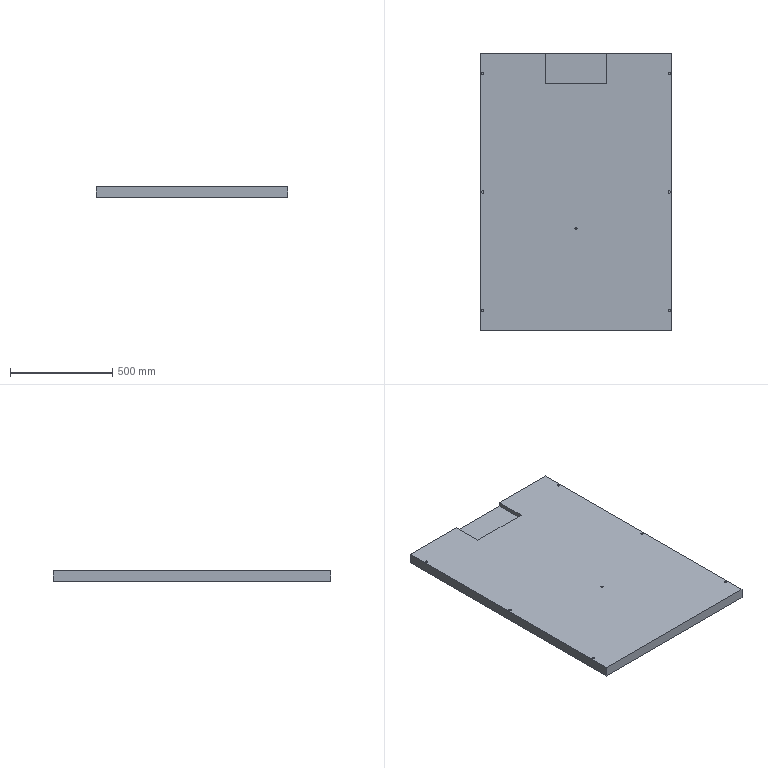Part | SolidWorks | features ICE 2, Extrusion 1 | 1 solid | 31 faces | box 940 x 1360 x 50 mm | volume 63007025 mm3 | plane 17 | cylinder 14 | commonest cylinder face diameters 11 x12 10 x2
STEP:
#1=CARTESIAN_POINT('',(-463.,-580.,30.));
#2=VERTEX_POINT('',#1);
#3=CARTESIAN_POINT('',(-452.,-580.,30.));
#4=VERTEX_POINT('',#3);
#5=CARTESIAN_POINT('',(-457.5,-580.,30.));
#6=DIRECTION('',(0.,0.,1.));
#7=DIRECTION('',(-1.,0.,0.));
#8=AXIS2_PLACEMENT_3D('',#5,#6,#7);
#9=CIRCLE('',#8,5.5);
#10=EDGE_CURVE('',#2,#4,#9,.T.);
#11=ORIENTED_EDGE('',*,*,#10,.F.);
#12=CARTESIAN_POINT('',(-463.,-580.,50.));
#13=VERTEX_POINT('',#12);
#14=CARTESIAN_POINT('',(-463.,-580.,30.));
#15=DIRECTION('',(0.,0.,1.));
#16=VECTOR('',#15,1000.);
#17=LINE('',#14,#16);
#18=EDGE_CURVE('',#2,#13,#17,.T.);
#19=ORIENTED_EDGE('',*,*,#18,.T.);
#20=CARTESIAN_POINT('',(-452.,-580.,50.));
#21=VERTEX_POINT('',#20);
#22=CARTESIAN_POINT('',(-457.5,-580.,50.));
#23=DIRECTION('',(0.,0.,1.));
#24=DIRECTION('',(-1.,0.,0.));
#25=AXIS2_PLACEMENT_3D('',#22,#23,#24);
#26=CIRCLE('',#25,5.5);
#27=EDGE_CURVE('',#13,#21,#26,.T.);
#28=ORIENTED_EDGE('',*,*,#27,.T.);
#29=CARTESIAN_POINT('',(-452.,-580.,30.));
#30=DIRECTION('',(0.,0.,1.));
#31=VECTOR('',#30,1000.);
#32=LINE('',#29,#31);
#33=EDGE_CURVE('',#4,#21,#32,.T.);
#34=ORIENTED_EDGE('',*,*,#33,.F.);
#35=EDGE_LOOP('',(#11,#19,#28,#34));
#36=FACE_OUTER_BOUND('',#35,.T.);
#37=CARTESIAN_POINT('',(-457.5,-580.,30.));
#38=DIRECTION('',(0.,0.,1.));
#39=DIRECTION('',(1.,0.,0.));
#40=AXIS2_PLACEMENT_3D('',#37,#38,#39);
#41=CYLINDRICAL_SURFACE('',#40,5.5);
#42=ADVANCED_FACE('',(#36),#41,.F.);
#43=CARTESIAN_POINT('',(-463.,0.,30.));
#44=VERTEX_POINT('',#43);
#45=CARTESIAN_POINT('',(-452.,0.,30.));
#46=VERTEX_POINT('',#45);
#47=CARTESIAN_POINT('',(-457.5,0.,30.));
#48=DIRECTION('',(0.,0.,1.));
#49=DIRECTION('',(-1.,0.,0.));
#50=AXIS2_PLACEMENT_3D('',#47,#48,#49);
#51=CIRCLE('',#50,5.5);
#52=EDGE_CURVE('',#44,#46,#51,.T.);
#53=ORIENTED_EDGE('',*,*,#52,.F.);
#54=CARTESIAN_POINT('',(-463.,0.,50.));
#55=VERTEX_POINT('',#54);
#56=CARTESIAN_POINT('',(-463.,0.,30.));
#57=DIRECTION('',(0.,0.,1.));
#58=VECTOR('',#57,1000.);
#59=LINE('',#56,#58);
#60=EDGE_CURVE('',#44,#55,#59,.T.);
#61=ORIENTED_EDGE('',*,*,#60,.T.);
#62=CARTESIAN_POINT('',(-452.,0.,50.));
#63=VERTEX_POINT('',#62);
#64=CARTESIAN_POINT('',(-457.5,0.,50.));
#65=DIRECTION('',(0.,0.,1.));
#66=DIRECTION('',(-1.,0.,0.));
#67=AXIS2_PLACEMENT_3D('',#64,#65,#66);
#68=CIRCLE('',#67,5.5);
#69=EDGE_CURVE('',#55,#63,#68,.T.);
#70=ORIENTED_EDGE('',*,*,#69,.T.);
#71=CARTESIAN_POINT('',(-452.,0.,30.));
#72=DIRECTION('',(0.,0.,1.));
#73=VECTOR('',#72,1000.);
#74=LINE('',#71,#73);
#75=EDGE_CURVE('',#46,#63,#74,.T.);
#76=ORIENTED_EDGE('',*,*,#75,.F.);
#77=EDGE_LOOP('',(#53,#61,#70,#76));
#78=FACE_OUTER_BOUND('',#77,.T.);
#79=CARTESIAN_POINT('',(-457.5,0.,30.));
#80=DIRECTION('',(0.,0.,1.));
#81=DIRECTION('',(1.,0.,0.));
#82=AXIS2_PLACEMENT_3D('',#79,#80,#81);
#83=CYLINDRICAL_SURFACE('',#82,5.5);
#84=ADVANCED_FACE('',(#78),#83,.F.);
#85=CARTESIAN_POINT('',(-463.,580.,30.));
#86=VERTEX_POINT('',#85);
#87=CARTESIAN_POINT('',(-452.,580.,30.));
#88=VERTEX_POINT('',#87);
#89=CARTESIAN_POINT('',(-457.5,580.,30.));
#90=DIRECTION('',(0.,0.,1.));
#91=DIRECTION('',(-1.,0.,0.));
#92=AXIS2_PLACEMENT_3D('',#89,#90,#91);
#93=CIRCLE('',#92,5.5);
#94=EDGE_CURVE('',#86,#88,#93,.T.);
#95=ORIENTED_EDGE('',*,*,#94,.F.);
#96=CARTESIAN_POINT('',(-463.,580.,50.));
#97=VERTEX_POINT('',#96);
#98=CARTESIAN_POINT('',(-463.,580.,30.));
#99=DIRECTION('',(0.,0.,1.));
#100=VECTOR('',#99,1000.);
#101=LINE('',#98,#100);
#102=EDGE_CURVE('',#86,#97,#101,.T.);
#103=ORIENTED_EDGE('',*,*,#102,.T.);
#104=CARTESIAN_POINT('',(-452.,580.,50.));
#105=VERTEX_POINT('',#104);
#106=CARTESIAN_POINT('',(-457.5,580.,50.));
#107=DIRECTION('',(0.,0.,1.));
#108=DIRECTION('',(-1.,0.,0.));
#109=AXIS2_PLACEMENT_3D('',#106,#107,#108);
#110=CIRCLE('',#109,5.5);
#111=EDGE_CURVE('',#97,#105,#110,.T.);
#112=ORIENTED_EDGE('',*,*,#111,.T.);
#113=CARTESIAN_POINT('',(-452.,580.,30.));
#114=DIRECTION('',(0.,0.,1.));
#115=VECTOR('',#114,1000.);
#116=LINE('',#113,#115);
#117=EDGE_CURVE('',#88,#105,#116,.T.);
#118=ORIENTED_EDGE('',*,*,#117,.F.);
#119=EDGE_LOOP('',(#95,#103,#112,#118));
#120=FACE_OUTER_BOUND('',#119,.T.);
#121=CARTESIAN_POINT('',(-457.5,580.,30.));
#122=DIRECTION('',(0.,0.,1.));
#123=DIRECTION('',(1.,0.,0.));
#124=AXIS2_PLACEMENT_3D('',#121,#122,#123);
#125=CYLINDRICAL_SURFACE('',#124,5.5);
#126=ADVANCED_FACE('',(#120),#125,.F.);
#127=CARTESIAN_POINT('',(452.,580.,30.));
#128=VERTEX_POINT('',#127);
#129=CARTESIAN_POINT('',(463.,580.,30.));
#130=VERTEX_POINT('',#129);
#131=CARTESIAN_POINT('',(457.5,580.,30.));
#132=DIRECTION('',(0.,0.,1.));
#133=DIRECTION('',(1.,0.,0.));
#134=AXIS2_PLACEMENT_3D('',#131,#132,#133);
#135=CIRCLE('',#134,5.5);
#136=EDGE_CURVE('',#128,#130,#135,.T.);
#137=ORIENTED_EDGE('',*,*,#136,.F.);
#138=CARTESIAN_POINT('',(452.,580.,50.));
#139=VERTEX_POINT('',#138);
#140=CARTESIAN_POINT('',(452.,580.,30.));
#141=DIRECTION('',(0.,0.,1.));
#142=VECTOR('',#141,1000.);
#143=LINE('',#140,#142);
#144=EDGE_CURVE('',#128,#139,#143,.T.);
#145=ORIENTED_EDGE('',*,*,#144,.T.);
#146=CARTESIAN_POINT('',(463.,580.,50.));
#147=VERTEX_POINT('',#146);
#148=CARTESIAN_POINT('',(457.5,580.,50.));
#149=DIRECTION('',(0.,0.,1.));
#150=DIRECTION('',(1.,0.,0.));
#151=AXIS2_PLACEMENT_3D('',#148,#149,#150);
#152=CIRCLE('',#151,5.5);
#153=EDGE_CURVE('',#139,#147,#152,.T.);
#154=ORIENTED_EDGE('',*,*,#153,.T.);
#155=CARTESIAN_POINT('',(463.,580.,30.));
#156=DIRECTION('',(0.,0.,1.));
#157=VECTOR('',#156,1000.);
#158=LINE('',#155,#157);
#159=EDGE_CURVE('',#130,#147,#158,.T.);
#160=ORIENTED_EDGE('',*,*,#159,.F.);
#161=EDGE_LOOP('',(#137,#145,#154,#160));
#162=FACE_OUTER_BOUND('',#161,.T.);
#163=CARTESIAN_POINT('',(457.5,580.,30.));
#164=DIRECTION('',(0.,0.,1.));
#165=DIRECTION('',(1.,0.,0.));
#166=AXIS2_PLACEMENT_3D('',#163,#164,#165);
#167=CYLINDRICAL_SURFACE('',#166,5.5);
#168=ADVANCED_FACE('',(#162),#167,.F.);
#169=CARTESIAN_POINT('',(452.,0.,30.));
#170=VERTEX_POINT('',#169);
#171=CARTESIAN_POINT('',(463.,0.,30.));
#172=VERTEX_POINT('',#171);
#173=CARTESIAN_POINT('',(457.5,0.,30.));
#174=DIRECTION('',(0.,0.,1.));
#175=DIRECTION('',(1.,0.,0.));
#176=AXIS2_PLACEMENT_3D('',#173,#174,#175);
#177=CIRCLE('',#176,5.5);
#178=EDGE_CURVE('',#170,#172,#177,.T.);
#179=ORIENTED_EDGE('',*,*,#178,.F.);
#180=CARTESIAN_POINT('',(452.,0.,50.));
#181=VERTEX_POINT('',#180);
#182=CARTESIAN_POINT('',(452.,0.,30.));
#183=DIRECTION('',(0.,0.,1.));
#184=VECTOR('',#183,1000.);
#185=LINE('',#182,#184);
#186=EDGE_CURVE('',#170,#181,#185,.T.);
#187=ORIENTED_EDGE('',*,*,#186,.T.);
#188=CARTESIAN_POINT('',(463.,0.,50.));
#189=VERTEX_POINT('',#188);
#190=CARTESIAN_POINT('',(457.5,0.,50.));
#191=DIRECTION('',(0.,0.,1.));
#192=DIRECTION('',(1.,0.,0.));
#193=AXIS2_PLACEMENT_3D('',#190,#191,#192);
#194=CIRCLE('',#193,5.5);
#195=EDGE_CURVE('',#181,#189,#194,.T.);
#196=ORIENTED_EDGE('',*,*,#195,.T.);
#197=CARTESIAN_POINT('',(463.,0.,30.));
#198=DIRECTION('',(0.,0.,1.));
#199=VECTOR('',#198,1000.);
#200=LINE('',#197,#199);
#201=EDGE_CURVE('',#172,#189,#200,.T.);
#202=ORIENTED_EDGE('',*,*,#201,.F.);
#203=EDGE_LOOP('',(#179,#187,#196,#202));
#204=FACE_OUTER_BOUND('',#203,.T.);
#205=CARTESIAN_POINT('',(457.5,0.,30.));
#206=DIRECTION('',(0.,0.,1.));
#207=DIRECTION('',(1.,0.,0.));
#208=AXIS2_PLACEMENT_3D('',#205,#206,#207);
#209=CYLINDRICAL_SURFACE('',#208,5.5);
#210=ADVANCED_FACE('',(#204),#209,.F.);
#211=CARTESIAN_POINT('',(452.,-580.,30.));
#212=VERTEX_POINT('',#211);
#213=CARTESIAN_POINT('',(463.,-580.,30.));
#214=VERTEX_POINT('',#213);
#215=CARTESIAN_POINT('',(457.5,-580.,30.));
#216=DIRECTION('',(0.,0.,1.));
#217=DIRECTION('',(1.,0.,0.));
#218=AXIS2_PLACEMENT_3D('',#215,#216,#217);
#219=CIRCLE('',#218,5.5);
#220=EDGE_CURVE('',#212,#214,#219,.T.);
#221=ORIENTED_EDGE('',*,*,#220,.F.);
#222=CARTESIAN_POINT('',(452.,-580.,50.));
#223=VERTEX_POINT('',#222);
#224=CARTESIAN_POINT('',(452.,-580.,30.));
#225=DIRECTION('',(0.,0.,1.));
#226=VECTOR('',#225,1000.);
#227=LINE('',#224,#226);
#228=EDGE_CURVE('',#212,#223,#227,.T.);
#229=ORIENTED_EDGE('',*,*,#228,.T.);
#230=CARTESIAN_POINT('',(463.,-580.,50.));
#231=VERTEX_POINT('',#230);
#232=CARTESIAN_POINT('',(457.5,-580.,50.));
#233=DIRECTION('',(0.,0.,1.));
#234=DIRECTION('',(1.,0.,0.));
#235=AXIS2_PLACEMENT_3D('',#232,#233,#234);
#236=CIRCLE('',#235,5.5);
#237=EDGE_CURVE('',#223,#231,#236,.T.);
#238=ORIENTED_EDGE('',*,*,#237,.T.);
#239=CARTESIAN_POINT('',(463.,-580.,30.));
#240=DIRECTION('',(0.,0.,1.));
#241=VECTOR('',#240,1000.);
#242=LINE('',#239,#241);
#243=EDGE_CURVE('',#214,#231,#242,.T.);
#244=ORIENTED_EDGE('',*,*,#243,.F.);
#245=EDGE_LOOP('',(#221,#229,#238,#244));
#246=FACE_OUTER_BOUND('',#245,.T.);
#247=CARTESIAN_POINT('',(457.5,-580.,30.));
#248=DIRECTION('',(0.,0.,1.));
#249=DIRECTION('',(1.,0.,0.));
#250=AXIS2_PLACEMENT_3D('',#247,#248,#249);
#251=CYLINDRICAL_SURFACE('',#250,5.5);
#252=ADVANCED_FACE('',(#246),#251,.F.);
#253=CARTESIAN_POINT('',(-5.,-180.,30.));
#254=VERTEX_POINT('',#253);
#255=CARTESIAN_POINT('',(5.,-180.,30.));
#256=VERTEX_POINT('',#255);
#257=CARTESIAN_POINT('',(0.,-180.,30.));
#258=DIRECTION('',(0.,0.,1.));
#259=DIRECTION('',(1.,0.,0.));
#260=AXIS2_PLACEMENT_3D('',#257,#258,#259);
#261=CIRCLE('',#260,5.);
#262=EDGE_CURVE('',#254,#256,#261,.T.);
#263=ORIENTED_EDGE('',*,*,#262,.F.);
#264=CARTESIAN_POINT('',(-5.,-180.,50.));
#265=VERTEX_POINT('',#264);
#266=CARTESIAN_POINT('',(-5.,-180.,30.));
#267=DIRECTION('',(0.,0.,1.));
#268=VECTOR('',#267,1000.);
#269=LINE('',#266,#268);
#270=EDGE_CURVE('',#254,#265,#269,.T.);
#271=ORIENTED_EDGE('',*,*,#270,.T.);
#272=CARTESIAN_POINT('',(5.,-180.,50.));
#273=VERTEX_POINT('',#272);
#274=CARTESIAN_POINT('',(0.,-180.,50.));
#275=DIRECTION('',(0.,0.,1.));
#276=DIRECTION('',(1.,0.,0.));
#277=AXIS2_PLACEMENT_3D('',#274,#275,#276);
#278=CIRCLE('',#277,5.);
#279=EDGE_CURVE('',#265,#273,#278,.T.);
#280=ORIENTED_EDGE('',*,*,#279,.T.);
#281=CARTESIAN_POINT('',(5.,-180.,30.));
#282=DIRECTION('',(0.,0.,1.));
#283=VECTOR('',#282,1000.);
#284=LINE('',#281,#283);
#285=EDGE_CURVE('',#256,#273,#284,.T.);
#286=ORIENTED_EDGE('',*,*,#285,.F.);
#287=EDGE_LOOP('',(#263,#271,#280,#286));
#288=FACE_OUTER_BOUND('',#287,.T.);
#289=CARTESIAN_POINT('',(0.,-180.,30.));
#290=DIRECTION('',(0.,0.,1.));
#291=DIRECTION('',(1.,0.,0.));
#292=AXIS2_PLACEMENT_3D('',#289,#290,#291);
#293=CYLINDRICAL_SURFACE('',#292,5.);
#294=ADVANCED_FACE('',(#288),#293,.F.);
#295=CARTESIAN_POINT('',(470.,-680.,0.));
#296=VERTEX_POINT('',#295);
#297=CARTESIAN_POINT('',(470.,680.,0.));
#298=VERTEX_POINT('',#297);
#299=CARTESIAN_POINT('',(470.,680.,0.));
#300=DIRECTION('',(0.,1.,0.));
#301=VECTOR('',#300,1000.);
#302=LINE('',#299,#301);
#303=EDGE_CURVE('',#296,#298,#302,.T.);
#304=ORIENTED_EDGE('',*,*,#303,.T.);
#305=CARTESIAN_POINT('',(470.,680.,50.));
#306=VERTEX_POINT('',#305);
#307=CARTESIAN_POINT('',(470.,680.,50.));
#308=DIRECTION('',(0.,0.,-1.));
#309=VECTOR('',#308,1000.);
#310=LINE('',#307,#309);
#311=EDGE_CURVE('',#306,#298,#310,.T.);
#312=ORIENTED_EDGE('',*,*,#311,.F.);
#313=CARTESIAN_POINT('',(470.,-680.,50.));
#314=VERTEX_POINT('',#313);
#315=CARTESIAN_POINT('',(470.,680.,50.));
#316=DIRECTION('',(0.,1.,0.));
#317=VECTOR('',#316,1000.);
#318=LINE('',#315,#317);
#319=EDGE_CURVE('',#314,#306,#318,.T.);
#320=ORIENTED_EDGE('',*,*,#319,.F.);
#321=CARTESIAN_POINT('',(470.,-680.,50.));
#322=DIRECTION('',(0.,0.,-1.));
#323=VECTOR('',#322,1000.);
#324=LINE('',#321,#323);
#325=EDGE_CURVE('',#314,#296,#324,.T.);
#326=ORIENTED_EDGE('',*,*,#325,.T.);
#327=EDGE_LOOP('',(#304,#312,#320,#326));
#328=FACE_OUTER_BOUND('',#327,.T.);
#329=CARTESIAN_POINT('',(470.,680.,50.));
#330=DIRECTION('',(-1.,0.,0.));
#331=DIRECTION('',(0.,-1.,0.));
#332=AXIS2_PLACEMENT_3D('',#329,#330,#331);
#333=PLANE('',#332);
#334=ADVANCED_FACE('',(#328),#333,.F.);
#335=CARTESIAN_POINT('',(150.,680.,30.));
#336=VERTEX_POINT('',#335);
#337=CARTESIAN_POINT('',(-150.,680.,30.));
#338=VERTEX_POINT('',#337);
#339=CARTESIAN_POINT('',(-470.,680.,30.));
#340=DIRECTION('',(-1.,0.,0.));
#341=VECTOR('',#340,1000.);
#342=LINE('',#339,#341);
#343=EDGE_CURVE('',#336,#338,#342,.T.);
#344=ORIENTED_EDGE('',*,*,#343,.F.);
#345=CARTESIAN_POINT('',(150.,680.,50.));
#346=VERTEX_POINT('',#345);
#347=CARTESIAN_POINT('',(150.,680.,50.));
#348=DIRECTION('',(0.,0.,1.));
#349=VECTOR('',#348,1000.);
#350=LINE('',#347,#349);
#351=EDGE_CURVE('',#336,#346,#350,.T.);
#352=ORIENTED_EDGE('',*,*,#351,.T.);
#353=CARTESIAN_POINT('',(-470.,680.,50.));
#354=DIRECTION('',(-1.,0.,0.));
#355=VECTOR('',#354,1000.);
#356=LINE('',#353,#355);
#357=EDGE_CURVE('',#306,#346,#356,.T.);
#358=ORIENTED_EDGE('',*,*,#357,.F.);
#359=ORIENTED_EDGE('',*,*,#311,.T.);
#360=CARTESIAN_POINT('',(-470.,680.,0.));
#361=VERTEX_POINT('',#360);
#362=CARTESIAN_POINT('',(-470.,680.,0.));
#363=DIRECTION('',(-1.,0.,0.));
#364=VECTOR('',#363,1000.);
#365=LINE('',#362,#364);
#366=EDGE_CURVE('',#298,#361,#365,.T.);
#367=ORIENTED_EDGE('',*,*,#366,.T.);
#368=CARTESIAN_POINT('',(-470.,680.,50.));
#369=VERTEX_POINT('',#368);
#370=CARTESIAN_POINT('',(-470.,680.,50.));
#371=DIRECTION('',(0.,0.,-1.));
#372=VECTOR('',#371,1000.);
#373=LINE('',#370,#372);
#374=EDGE_CURVE('',#369,#361,#373,.T.);
#375=ORIENTED_EDGE('',*,*,#374,.F.);
#376=CARTESIAN_POINT('',(-150.,680.,50.));
#377=VERTEX_POINT('',#376);
#378=CARTESIAN_POINT('',(-470.,680.,50.));
#379=DIRECTION('',(-1.,0.,0.));
#380=VECTOR('',#379,1000.);
#381=LINE('',#378,#380);
#382=EDGE_CURVE('',#377,#369,#381,.T.);
#383=ORIENTED_EDGE('',*,*,#382,.F.);
#384=CARTESIAN_POINT('',(-150.,680.,50.));
#385=DIRECTION('',(0.,0.,-1.));
#386=VECTOR('',#385,1000.);
#387=LINE('',#384,#386);
#388=EDGE_CURVE('',#377,#338,#387,.T.);
#389=ORIENTED_EDGE('',*,*,#388,.T.);
#390=EDGE_LOOP('',(#344,#352,#358,#359,#367,#375,#383,#389));
#391=FACE_OUTER_BOUND('',#390,.T.);
#392=CARTESIAN_POINT('',(-470.,680.,50.));
#393=DIRECTION('',(0.,-1.,0.));
#394=DIRECTION('',(0.,0.,-1.));
#395=AXIS2_PLACEMENT_3D('',#392,#393,#394);
#396=PLANE('',#395);
#397=ADVANCED_FACE('',(#391),#396,.F.);
#398=CARTESIAN_POINT('',(-470.,-680.,0.));
#399=VERTEX_POINT('',#398);
#400=CARTESIAN_POINT('',(-470.,680.,0.));
#401=DIRECTION('',(0.,-1.,0.));
#402=VECTOR('',#401,1000.);
#403=LINE('',#400,#402);
#404=EDGE_CURVE('',#361,#399,#403,.T.);
#405=ORIENTED_EDGE('',*,*,#404,.T.);
#406=CARTESIAN_POINT('',(-470.,-680.,50.));
#407=VERTEX_POINT('',#406);
#408=CARTESIAN_POINT('',(-470.,-680.,50.));
#409=DIRECTION('',(0.,0.,-1.));
#410=VECTOR('',#409,1000.);
#411=LINE('',#408,#410);
#412=EDGE_CURVE('',#407,#399,#411,.T.);
#413=ORIENTED_EDGE('',*,*,#412,.F.);
#414=CARTESIAN_POINT('',(-470.,680.,50.));
#415=DIRECTION('',(0.,-1.,0.));
#416=VECTOR('',#415,1000.);
#417=LINE('',#414,#416);
#418=EDGE_CURVE('',#369,#407,#417,.T.);
#419=ORIENTED_EDGE('',*,*,#418,.F.);
#420=ORIENTED_EDGE('',*,*,#374,.T.);
#421=EDGE_LOOP('',(#405,#413,#419,#420));
#422=FACE_OUTER_BOUND('',#421,.T.);
#423=CARTESIAN_POINT('',(-470.,680.,50.));
#424=DIRECTION('',(1.,0.,0.));
#425=DIRECTION('',(0.,1.,0.));
#426=AXIS2_PLACEMENT_3D('',#423,#424,#425);
#427=PLANE('',#426);
#428=ADVANCED_FACE('',(#422),#427,.F.);
#429=CARTESIAN_POINT('',(-470.,-680.,0.));
#430=DIRECTION('',(1.,0.,0.));
#431=VECTOR('',#430,1000.);
#432=LINE('',#429,#431);
#433=EDGE_CURVE('',#399,#296,#432,.T.);
#434=ORIENTED_EDGE('',*,*,#433,.T.);
#435=ORIENTED_EDGE('',*,*,#325,.F.);
#436=CARTESIAN_POINT('',(-470.,-680.,50.));
#437=DIRECTION('',(1.,0.,0.));
#438=VECTOR('',#437,1000.);
#439=LINE('',#436,#438);
#440=EDGE_CURVE('',#407,#314,#439,.T.);
#441=ORIENTED_EDGE('',*,*,#440,.F.);
#442=ORIENTED_EDGE('',*,*,#412,.T.);
#443=EDGE_LOOP('',(#434,#435,#441,#442));
#444=FACE_OUTER_BOUND('',#443,.T.);
#445=CARTESIAN_POINT('',(-470.,-680.,50.));
#446=DIRECTION('',(0.,1.,0.));
#447=DIRECTION('',(0.,0.,1.));
#448=AXIS2_PLACEMENT_3D('',#445,#446,#447);
#449=PLANE('',#448);
#450=ADVANCED_FACE('',(#444),#449,.F.);
#451=CARTESIAN_POINT('',(-457.5,-580.,50.));
#452=DIRECTION('',(0.,0.,1.));
#453=DIRECTION('',(-1.,0.,0.));
#454=AXIS2_PLACEMENT_3D('',#451,#452,#453);
#455=CIRCLE('',#454,5.5);
#456=EDGE_CURVE('',#21,#13,#455,.T.);
#457=ORIENTED_EDGE('',*,*,#456,.F.);
#458=ORIENTED_EDGE('',*,*,#27,.F.);
#459=EDGE_LOOP('',(#457,#458));
#460=FACE_BOUND('',#459,.T.);
#461=CARTESIAN_POINT('',(-457.5,0.,50.));
#462=DIRECTION('',(0.,0.,1.));
#463=DIRECTION('',(-1.,0.,0.));
#464=AXIS2_PLACEMENT_3D('',#461,#462,#463);
#465=CIRCLE('',#464,5.5);
#466=EDGE_CURVE('',#63,#55,#465,.T.);
#467=ORIENTED_EDGE('',*,*,#466,.F.);
#468=ORIENTED_EDGE('',*,*,#69,.F.);
#469=EDGE_LOOP('',(#467,#468));
#470=FACE_BOUND('',#469,.T.);
#471=CARTESIAN_POINT('',(-457.5,580.,50.));
#472=DIRECTION('',(0.,0.,1.));
#473=DIRECTION('',(-1.,0.,0.));
#474=AXIS2_PLACEMENT_3D('',#471,#472,#473);
#475=CIRCLE('',#474,5.5);
#476=EDGE_CURVE('',#105,#97,#475,.T.);
#477=ORIENTED_EDGE('',*,*,#476,.F.);
#478=ORIENTED_EDGE('',*,*,#111,.F.);
#479=EDGE_LOOP('',(#477,#478));
#480=FACE_BOUND('',#479,.T.);
#481=CARTESIAN_POINT('',(457.5,580.,50.));
#482=DIRECTION('',(0.,0.,1.));
#483=DIRECTION('',(1.,0.,0.));
#484=AXIS2_PLACEMENT_3D('',#481,#482,#483);
#485=CIRCLE('',#484,5.5);
#486=EDGE_CURVE('',#147,#139,#485,.T.);
#487=ORIENTED_EDGE('',*,*,#486,.F.);
#488=ORIENTED_EDGE('',*,*,#153,.F.);
#489=EDGE_LOOP('',(#487,#488));
#490=FACE_BOUND('',#489,.T.);
#491=CARTESIAN_POINT('',(457.5,0.,50.));
#492=DIRECTION('',(0.,0.,1.));
#493=DIRECTION('',(1.,0.,0.));
#494=AXIS2_PLACEMENT_3D('',#491,#492,#493);
#495=CIRCLE('',#494,5.5);
#496=EDGE_CURVE('',#189,#181,#495,.T.);
#497=ORIENTED_EDGE('',*,*,#496,.F.);
#498=ORIENTED_EDGE('',*,*,#195,.F.);
#499=EDGE_LOOP('',(#497,#498));
#500=FACE_BOUND('',#499,.T.);
#501=CARTESIAN_POINT('',(457.5,-580.,50.));
#502=DIRECTION('',(0.,0.,1.));
#503=DIRECTION('',(1.,0.,0.));
#504=AXIS2_PLACEMENT_3D('',#501,#502,#503);
#505=CIRCLE('',#504,5.5);
#506=EDGE_CURVE('',#231,#223,#505,.T.);
#507=ORIENTED_EDGE('',*,*,#506,.F.);
#508=ORIENTED_EDGE('',*,*,#237,.F.);
#509=EDGE_LOOP('',(#507,#508));
#510=FACE_BOUND('',#509,.T.);
#511=CARTESIAN_POINT('',(0.,-180.,50.));
#512=DIRECTION('',(0.,0.,1.));
#513=DIRECTION('',(1.,0.,0.));
#514=AXIS2_PLACEMENT_3D('',#511,#512,#513);
#515=CIRCLE('',#514,5.);
#516=EDGE_CURVE('',#273,#265,#515,.T.);
#517=ORIENTED_EDGE('',*,*,#516,.F.);
#518=ORIENTED_EDGE('',*,*,#279,.F.);
#519=EDGE_LOOP('',(#517,#518));
#520=FACE_BOUND('',#519,.T.);
#521=CARTESIAN_POINT('',(150.,530.,50.));
#522=VERTEX_POINT('',#521);
#523=CARTESIAN_POINT('',(150.,830.,50.));
#524=DIRECTION('',(0.,1.,0.));
#525=VECTOR('',#524,1000.);
#526=LINE('',#523,#525);
#527=EDGE_CURVE('',#522,#346,#526,.T.);
#528=ORIENTED_EDGE('',*,*,#527,.F.);
#529=CARTESIAN_POINT('',(-150.,530.,50.));
#530=VERTEX_POINT('',#529);
#531=CARTESIAN_POINT('',(-150.,530.,50.));
#532=DIRECTION('',(1.,0.,0.));
#533=VECTOR('',#532,1000.);
#534=LINE('',#531,#533);
#535=EDGE_CURVE('',#530,#522,#534,.T.);
#536=ORIENTED_EDGE('',*,*,#535,.F.);
#537=CARTESIAN_POINT('',(-150.,0.,50.));
#538=DIRECTION('',(0.,-1.,0.));
#539=VECTOR('',#538,1000.);
#540=LINE('',#537,#539);
#541=EDGE_CURVE('',#377,#530,#540,.T.);
#542=ORIENTED_EDGE('',*,*,#541,.F.);
#543=ORIENTED_EDGE('',*,*,#382,.T.);
#544=ORIENTED_EDGE('',*,*,#418,.T.);
#545=ORIENTED_EDGE('',*,*,#440,.T.);
#546=ORIENTED_EDGE('',*,*,#319,.T.);
#547=ORIENTED_EDGE('',*,*,#357,.T.);
#548=EDGE_LOOP('',(#528,#536,#542,#543,#544,#545,#546,#547));
#549=FACE_OUTER_BOUND('',#548,.T.);
#550=CARTESIAN_POINT('',(0.,0.,50.));
#551=DIRECTION('',(0.,0.,1.));
#552=DIRECTION('',(1.,0.,0.));
#553=AXIS2_PLACEMENT_3D('',#550,#551,#552);
#554=PLANE('',#553);
#555=ADVANCED_FACE('',(#460,#470,#480,#490,#500,#510,#520,#549),#554,.T.);
#556=ORIENTED_EDGE('',*,*,#303,.F.);
#557=ORIENTED_EDGE('',*,*,#433,.F.);
#558=ORIENTED_EDGE('',*,*,#404,.F.);
#559=ORIENTED_EDGE('',*,*,#366,.F.);
#560=EDGE_LOOP('',(#556,#557,#558,#559));
#561=FACE_OUTER_BOUND('',#560,.T.);
#562=CARTESIAN_POINT('',(0.,0.,0.));
#563=DIRECTION('',(0.,0.,1.));
#564=DIRECTION('',(1.,0.,0.));
#565=AXIS2_PLACEMENT_3D('',#562,#563,#564);
#566=PLANE('',#565);
#567=ADVANCED_FACE('',(#561),#566,.F.);
#568=ORIENTED_EDGE('',*,*,#343,.T.);
#569=CARTESIAN_POINT('',(-150.,530.,30.));
#570=VERTEX_POINT('',#569);
#571=CARTESIAN_POINT('',(-150.,830.,30.));
#572=DIRECTION('',(0.,-1.,0.));
#573=VECTOR('',#572,1000.);
#574=LINE('',#571,#573);
#575=EDGE_CURVE('',#338,#570,#574,.T.);
#576=ORIENTED_EDGE('',*,*,#575,.T.);
#577=CARTESIAN_POINT('',(150.,530.,30.));
#578=VERTEX_POINT('',#577);
#579=CARTESIAN_POINT('',(-150.,530.,30.));
#580=DIRECTION('',(1.,0.,0.));
#581=VECTOR('',#580,1000.);
#582=LINE('',#579,#581);
#583=EDGE_CURVE('',#570,#578,#582,.T.);
#584=ORIENTED_EDGE('',*,*,#583,.T.);
#585=CARTESIAN_POINT('',(150.,830.,30.));
#586=DIRECTION('',(0.,1.,0.));
#587=VECTOR('',#586,1000.);
#588=LINE('',#585,#587);
#589=EDGE_CURVE('',#578,#336,#588,.T.);
#590=ORIENTED_EDGE('',*,*,#589,.T.);
#591=EDGE_LOOP('',(#568,#576,#584,#590));
#592=FACE_OUTER_BOUND('',#591,.T.);
#593=CARTESIAN_POINT('',(0.,0.,30.));
#594=DIRECTION('',(0.,0.,1.));
#595=DIRECTION('',(1.,0.,0.));
#596=AXIS2_PLACEMENT_3D('',#593,#594,#595);
#597=PLANE('',#596);
#598=ADVANCED_FACE('',(#592),#597,.T.);
#599=ORIENTED_EDGE('',*,*,#589,.F.);
#600=CARTESIAN_POINT('',(150.,530.,30.));
#601=DIRECTION('',(0.,0.,1.));
#602=VECTOR('',#601,1000.);
#603=LINE('',#600,#602);
#604=EDGE_CURVE('',#578,#522,#603,.T.);
#605=ORIENTED_EDGE('',*,*,#604,.T.);
#606=ORIENTED_EDGE('',*,*,#527,.T.);
#607=ORIENTED_EDGE('',*,*,#351,.F.);
#608=EDGE_LOOP('',(#599,#605,#606,#607));
#609=FACE_OUTER_BOUND('',#608,.T.);
#610=CARTESIAN_POINT('',(150.,830.,30.));
#611=DIRECTION('',(1.,0.,0.));
#612=DIRECTION('',(0.,1.,0.));
#613=AXIS2_PLACEMENT_3D('',#610,#611,#612);
#614=PLANE('',#613);
#615=ADVANCED_FACE('',(#609),#614,.F.);
#616=ORIENTED_EDGE('',*,*,#541,.T.);
#617=CARTESIAN_POINT('',(-150.,530.,30.));
#618=DIRECTION('',(0.,0.,1.));
#619=VECTOR('',#618,1000.);
#620=LINE('',#617,#619);
#621=EDGE_CURVE('',#570,#530,#620,.T.);
#622=ORIENTED_EDGE('',*,*,#621,.F.);
#623=ORIENTED_EDGE('',*,*,#575,.F.);
#624=ORIENTED_EDGE('',*,*,#388,.F.);
#625=EDGE_LOOP('',(#616,#622,#623,#624));
#626=FACE_OUTER_BOUND('',#625,.T.);
#627=CARTESIAN_POINT('',(-150.,830.,30.));
#628=DIRECTION('',(-1.,0.,0.));
#629=DIRECTION('',(0.,-1.,0.));
#630=AXIS2_PLACEMENT_3D('',#627,#628,#629);
#631=PLANE('',#630);
#632=ADVANCED_FACE('',(#626),#631,.F.);
#633=ORIENTED_EDGE('',*,*,#535,.T.);
#634=ORIENTED_EDGE('',*,*,#604,.F.);
#635=ORIENTED_EDGE('',*,*,#583,.F.);
#636=ORIENTED_EDGE('',*,*,#621,.T.);
#637=EDGE_LOOP('',(#633,#634,#635,#636));
#638=FACE_OUTER_BOUND('',#637,.T.);
#639=CARTESIAN_POINT('',(-150.,530.,30.));
#640=DIRECTION('',(0.,-1.,0.));
#641=DIRECTION('',(0.,0.,-1.));
#642=AXIS2_PLACEMENT_3D('',#639,#640,#641);
#643=PLANE('',#642);
#644=ADVANCED_FACE('',(#638),#643,.F.);
#645=ORIENTED_EDGE('',*,*,#270,.F.);
#646=CARTESIAN_POINT('',(0.,-180.,30.));
#647=DIRECTION('',(0.,0.,1.));
#648=DIRECTION('',(1.,0.,0.));
#649=AXIS2_PLACEMENT_3D('',#646,#647,#648);
#650=CIRCLE('',#649,5.);
#651=EDGE_CURVE('',#256,#254,#650,.T.);
#652=ORIENTED_EDGE('',*,*,#651,.F.);
#653=ORIENTED_EDGE('',*,*,#285,.T.);
#654=ORIENTED_EDGE('',*,*,#516,.T.);
#655=EDGE_LOOP('',(#645,#652,#653,#654));
#656=FACE_OUTER_BOUND('',#655,.T.);
#657=CARTESIAN_POINT('',(0.,-180.,30.));
#658=DIRECTION('',(0.,0.,1.));
#659=DIRECTION('',(1.,0.,0.));
#660=AXIS2_PLACEMENT_3D('',#657,#658,#659);
#661=CYLINDRICAL_SURFACE('',#660,5.);
#662=ADVANCED_FACE('',(#656),#661,.F.);
#663=ORIENTED_EDGE('',*,*,#651,.T.);
#664=ORIENTED_EDGE('',*,*,#262,.T.);
#665=EDGE_LOOP('',(#663,#664));
#666=FACE_OUTER_BOUND('',#665,.T.);
#667=CARTESIAN_POINT('',(0.,-180.,30.));
#668=DIRECTION('',(0.,0.,1.));
#669=DIRECTION('',(1.,0.,0.));
#670=AXIS2_PLACEMENT_3D('',#667,#668,#669);
#671=PLANE('',#670);
#672=ADVANCED_FACE('',(#666),#671,.T.);
#673=ORIENTED_EDGE('',*,*,#228,.F.);
#674=CARTESIAN_POINT('',(457.5,-580.,30.));
#675=DIRECTION('',(0.,0.,1.));
#676=DIRECTION('',(1.,0.,0.));
#677=AXIS2_PLACEMENT_3D('',#674,#675,#676);
#678=CIRCLE('',#677,5.5);
#679=EDGE_CURVE('',#214,#212,#678,.T.);
#680=ORIENTED_EDGE('',*,*,#679,.F.);
#681=ORIENTED_EDGE('',*,*,#243,.T.);
#682=ORIENTED_EDGE('',*,*,#506,.T.);
#683=EDGE_LOOP('',(#673,#680,#681,#682));
#684=FACE_OUTER_BOUND('',#683,.T.);
#685=CARTESIAN_POINT('',(457.5,-580.,30.));
#686=DIRECTION('',(0.,0.,1.));
#687=DIRECTION('',(1.,0.,0.));
#688=AXIS2_PLACEMENT_3D('',#685,#686,#687);
#689=CYLINDRICAL_SURFACE('',#688,5.5);
#690=ADVANCED_FACE('',(#684),#689,.F.);
#691=ORIENTED_EDGE('',*,*,#679,.T.);
#692=ORIENTED_EDGE('',*,*,#220,.T.);
#693=EDGE_LOOP('',(#691,#692));
#694=FACE_OUTER_BOUND('',#693,.T.);
#695=CARTESIAN_POINT('',(457.5,-580.,30.));
#696=DIRECTION('',(0.,0.,1.));
#697=DIRECTION('',(1.,0.,0.));
#698=AXIS2_PLACEMENT_3D('',#695,#696,#697);
#699=PLANE('',#698);
#700=ADVANCED_FACE('',(#694),#699,.T.);
#701=ORIENTED_EDGE('',*,*,#186,.F.);
#702=CARTESIAN_POINT('',(457.5,0.,30.));
#703=DIRECTION('',(0.,0.,1.));
#704=DIRECTION('',(1.,0.,0.));
#705=AXIS2_PLACEMENT_3D('',#702,#703,#704);
#706=CIRCLE('',#705,5.5);
#707=EDGE_CURVE('',#172,#170,#706,.T.);
#708=ORIENTED_EDGE('',*,*,#707,.F.);
#709=ORIENTED_EDGE('',*,*,#201,.T.);
#710=ORIENTED_EDGE('',*,*,#496,.T.);
#711=EDGE_LOOP('',(#701,#708,#709,#710));
#712=FACE_OUTER_BOUND('',#711,.T.);
#713=CARTESIAN_POINT('',(457.5,0.,30.));
#714=DIRECTION('',(0.,0.,1.));
#715=DIRECTION('',(1.,0.,0.));
#716=AXIS2_PLACEMENT_3D('',#713,#714,#715);
#717=CYLINDRICAL_SURFACE('',#716,5.5);
#718=ADVANCED_FACE('',(#712),#717,.F.);
#719=ORIENTED_EDGE('',*,*,#707,.T.);
#720=ORIENTED_EDGE('',*,*,#178,.T.);
#721=EDGE_LOOP('',(#719,#720));
#722=FACE_OUTER_BOUND('',#721,.T.);
#723=CARTESIAN_POINT('',(457.5,0.,30.));
#724=DIRECTION('',(0.,0.,1.));
#725=DIRECTION('',(1.,0.,0.));
#726=AXIS2_PLACEMENT_3D('',#723,#724,#725);
#727=PLANE('',#726);
#728=ADVANCED_FACE('',(#722),#727,.T.);
#729=ORIENTED_EDGE('',*,*,#144,.F.);
#730=CARTESIAN_POINT('',(457.5,580.,30.));
#731=DIRECTION('',(0.,0.,1.));
#732=DIRECTION('',(1.,0.,0.));
#733=AXIS2_PLACEMENT_3D('',#730,#731,#732);
#734=CIRCLE('',#733,5.5);
#735=EDGE_CURVE('',#130,#128,#734,.T.);
#736=ORIENTED_EDGE('',*,*,#735,.F.);
#737=ORIENTED_EDGE('',*,*,#159,.T.);
#738=ORIENTED_EDGE('',*,*,#486,.T.);
#739=EDGE_LOOP('',(#729,#736,#737,#738));
#740=FACE_OUTER_BOUND('',#739,.T.);
#741=CARTESIAN_POINT('',(457.5,580.,30.));
#742=DIRECTION('',(0.,0.,1.));
#743=DIRECTION('',(1.,0.,0.));
#744=AXIS2_PLACEMENT_3D('',#741,#742,#743);
#745=CYLINDRICAL_SURFACE('',#744,5.5);
#746=ADVANCED_FACE('',(#740),#745,.F.);
#747=ORIENTED_EDGE('',*,*,#735,.T.);
#748=ORIENTED_EDGE('',*,*,#136,.T.);
#749=EDGE_LOOP('',(#747,#748));
#750=FACE_OUTER_BOUND('',#749,.T.);
#751=CARTESIAN_POINT('',(457.5,580.,30.));
#752=DIRECTION('',(0.,0.,1.));
#753=DIRECTION('',(1.,0.,0.));
#754=AXIS2_PLACEMENT_3D('',#751,#752,#753);
#755=PLANE('',#754);
#756=ADVANCED_FACE('',(#750),#755,.T.);
#757=ORIENTED_EDGE('',*,*,#102,.F.);
#758=CARTESIAN_POINT('',(-457.5,580.,30.));
#759=DIRECTION('',(0.,0.,1.));
#760=DIRECTION('',(-1.,0.,0.));
#761=AXIS2_PLACEMENT_3D('',#758,#759,#760);
#762=CIRCLE('',#761,5.5);
#763=EDGE_CURVE('',#88,#86,#762,.T.);
#764=ORIENTED_EDGE('',*,*,#763,.F.);
#765=ORIENTED_EDGE('',*,*,#117,.T.);
#766=ORIENTED_EDGE('',*,*,#476,.T.);
#767=EDGE_LOOP('',(#757,#764,#765,#766));
#768=FACE_OUTER_BOUND('',#767,.T.);
#769=CARTESIAN_POINT('',(-457.5,580.,30.));
#770=DIRECTION('',(0.,0.,1.));
#771=DIRECTION('',(1.,0.,0.));
#772=AXIS2_PLACEMENT_3D('',#769,#770,#771);
#773=CYLINDRICAL_SURFACE('',#772,5.5);
#774=ADVANCED_FACE('',(#768),#773,.F.);
#775=ORIENTED_EDGE('',*,*,#763,.T.);
#776=ORIENTED_EDGE('',*,*,#94,.T.);
#777=EDGE_LOOP('',(#775,#776));
#778=FACE_OUTER_BOUND('',#777,.T.);
#779=CARTESIAN_POINT('',(-457.5,580.,30.));
#780=DIRECTION('',(0.,0.,-1.));
#781=DIRECTION('',(-1.,0.,0.));
#782=AXIS2_PLACEMENT_3D('',#779,#780,#781);
#783=PLANE('',#782);
#784=ADVANCED_FACE('',(#778),#783,.F.);
#785=ORIENTED_EDGE('',*,*,#60,.F.);
#786=CARTESIAN_POINT('',(-457.5,0.,30.));
#787=DIRECTION('',(0.,0.,1.));
#788=DIRECTION('',(-1.,0.,0.));
#789=AXIS2_PLACEMENT_3D('',#786,#787,#788);
#790=CIRCLE('',#789,5.5);
#791=EDGE_CURVE('',#46,#44,#790,.T.);
#792=ORIENTED_EDGE('',*,*,#791,.F.);
#793=ORIENTED_EDGE('',*,*,#75,.T.);
#794=ORIENTED_EDGE('',*,*,#466,.T.);
#795=EDGE_LOOP('',(#785,#792,#793,#794));
#796=FACE_OUTER_BOUND('',#795,.T.);
#797=CARTESIAN_POINT('',(-457.5,0.,30.));
#798=DIRECTION('',(0.,0.,1.));
#799=DIRECTION('',(1.,0.,0.));
#800=AXIS2_PLACEMENT_3D('',#797,#798,#799);
#801=CYLINDRICAL_SURFACE('',#800,5.5);
#802=ADVANCED_FACE('',(#796),#801,.F.);
#803=ORIENTED_EDGE('',*,*,#791,.T.);
#804=ORIENTED_EDGE('',*,*,#52,.T.);
#805=EDGE_LOOP('',(#803,#804));
#806=FACE_OUTER_BOUND('',#805,.T.);
#807=CARTESIAN_POINT('',(-457.5,0.,30.));
#808=DIRECTION('',(0.,0.,-1.));
#809=DIRECTION('',(-1.,0.,0.));
#810=AXIS2_PLACEMENT_3D('',#807,#808,#809);
#811=PLANE('',#810);
#812=ADVANCED_FACE('',(#806),#811,.F.);
#813=ORIENTED_EDGE('',*,*,#18,.F.);
#814=CARTESIAN_POINT('',(-457.5,-580.,30.));
#815=DIRECTION('',(0.,0.,1.));
#816=DIRECTION('',(-1.,0.,0.));
#817=AXIS2_PLACEMENT_3D('',#814,#815,#816);
#818=CIRCLE('',#817,5.5);
#819=EDGE_CURVE('',#4,#2,#818,.T.);
#820=ORIENTED_EDGE('',*,*,#819,.F.);
#821=ORIENTED_EDGE('',*,*,#33,.T.);
#822=ORIENTED_EDGE('',*,*,#456,.T.);
#823=EDGE_LOOP('',(#813,#820,#821,#822));
#824=FACE_OUTER_BOUND('',#823,.T.);
#825=CARTESIAN_POINT('',(-457.5,-580.,30.));
#826=DIRECTION('',(0.,0.,1.));
#827=DIRECTION('',(1.,0.,0.));
#828=AXIS2_PLACEMENT_3D('',#825,#826,#827);
#829=CYLINDRICAL_SURFACE('',#828,5.5);
#830=ADVANCED_FACE('',(#824),#829,.F.);
#831=ORIENTED_EDGE('',*,*,#819,.T.);
#832=ORIENTED_EDGE('',*,*,#10,.T.);
#833=EDGE_LOOP('',(#831,#832));
#834=FACE_OUTER_BOUND('',#833,.T.);
#835=CARTESIAN_POINT('',(-457.5,-580.,30.));
#836=DIRECTION('',(0.,0.,-1.));
#837=DIRECTION('',(-1.,0.,0.));
#838=AXIS2_PLACEMENT_3D('',#835,#836,#837);
#839=PLANE('',#838);
#840=ADVANCED_FACE('',(#834),#839,.F.);
#841=CLOSED_SHELL('',(#42,#84,#126,#168,#210,#252,#294,#334,#397,#428,#450,#555,#567,#598,#615,#632,#644,#662,#672,#690,#700,#718,#728,#746,#756,#774,#784,#802,#812,#830,#840));
#842=MANIFOLD_SOLID_BREP('',#841);
#843=CARTESIAN_POINT('',(0.,0.,0.));
#844=DIRECTION('',(0.,0.,1.));
#845=DIRECTION('',(1.,0.,0.));
#846=AXIS2_PLACEMENT_3D('',#843,#844,#845);
#847=(LENGTH_UNIT()NAMED_UNIT(*)SI_UNIT(.MILLI.,.METRE.));
#848=UNCERTAINTY_MEASURE_WITH_UNIT(LENGTH_MEASURE(0.00001),#847,'','');
#849=(NAMED_UNIT(*)PLANE_ANGLE_UNIT()SI_UNIT($,.RADIAN.));
#850=(NAMED_UNIT(*)SI_UNIT($,.STERADIAN.)SOLID_ANGLE_UNIT());
#851=(GEOMETRIC_REPRESENTATION_CONTEXT(3)GLOBAL_UNCERTAINTY_ASSIGNED_CONTEXT((#848))GLOBAL_UNIT_ASSIGNED_CONTEXT((#847,#849,#850))REPRESENTATION_CONTEXT('',''));
#852=ADVANCED_BREP_SHAPE_REPRESENTATION('',(#842,#846),#851);